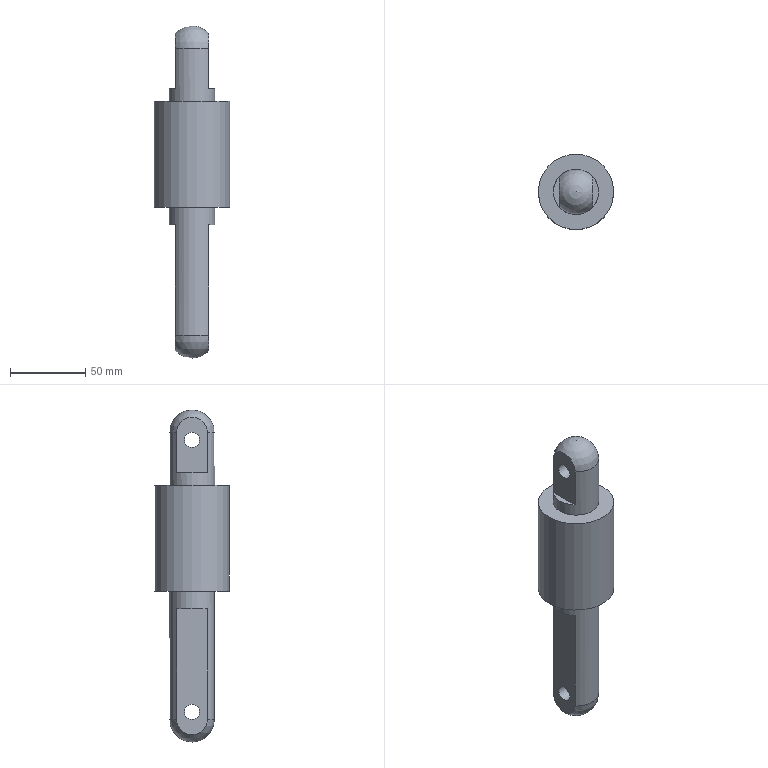Part | NX | features DATUM_CSYS 6, EXTRUDE 5, SKETCH 5, BLEND 2 | 1 solid | 17 faces | box 50 x 50 x 220 mm | volume 220357 mm3 | plane 10 | cylinder 5 | sphere 2 | commonest cylinder face diameters 10 x2 30 x2 50 x1
STEP:
#1=CARTESIAN_POINT('',(15.,0.,100.));
#2=VERTEX_POINT('',#1);
#3=CARTESIAN_POINT('',(0.,0.,100.));
#4=DIRECTION('',(0.,0.,1.));
#5=DIRECTION('',(1.,0.,0.));
#6=AXIS2_PLACEMENT_3D('',#3,#4,#5);
#7=CIRCLE('',#6,15.);
#8=EDGE_CURVE('',#2,#2,#7,.T.);
#9=ORIENTED_EDGE('',*,*,#8,.F.);
#10=EDGE_LOOP('',(#9));
#11=FACE_BOUND('',#10,.T.);
#12=CARTESIAN_POINT('',(11.,10.198,15.));
#13=VERTEX_POINT('',#12);
#14=CARTESIAN_POINT('',(11.,10.198,88.444));
#15=VERTEX_POINT('',#14);
#16=CARTESIAN_POINT('',(11.,10.198,100.));
#17=DIRECTION('',(0.,0.,-1.));
#18=VECTOR('',#17,1000.);
#19=LINE('',#16,#18);
#20=EDGE_CURVE('',#13,#15,#19,.F.);
#21=ORIENTED_EDGE('',*,*,#20,.F.);
#22=CARTESIAN_POINT('',(-11.,10.198,15.));
#23=VERTEX_POINT('',#22);
#24=CARTESIAN_POINT('',(0.,0.,15.));
#25=DIRECTION('',(0.,0.,-1.));
#26=DIRECTION('',(-1.,0.,0.));
#27=AXIS2_PLACEMENT_3D('',#24,#25,#26);
#28=CIRCLE('',#27,15.);
#29=EDGE_CURVE('',#13,#23,#28,.F.);
#30=ORIENTED_EDGE('',*,*,#29,.T.);
#31=CARTESIAN_POINT('',(-11.,10.198,88.444));
#32=VERTEX_POINT('',#31);
#33=CARTESIAN_POINT('',(-11.,10.198,100.));
#34=DIRECTION('',(0.,0.,-1.));
#35=VECTOR('',#34,1000.);
#36=LINE('',#33,#35);
#37=EDGE_CURVE('',#32,#23,#36,.T.);
#38=ORIENTED_EDGE('',*,*,#37,.F.);
#39=CARTESIAN_POINT('',(-11.,-10.198,88.444));
#40=VERTEX_POINT('',#39);
#41=CARTESIAN_POINT('',(0.,0.,88.444));
#42=DIRECTION('',(0.,0.,-1.));
#43=DIRECTION('',(-1.,0.,0.));
#44=AXIS2_PLACEMENT_3D('',#41,#42,#43);
#45=CIRCLE('',#44,15.);
#46=EDGE_CURVE('',#40,#32,#45,.T.);
#47=ORIENTED_EDGE('',*,*,#46,.F.);
#48=CARTESIAN_POINT('',(-11.,-10.198,15.));
#49=VERTEX_POINT('',#48);
#50=CARTESIAN_POINT('',(-11.,-10.198,100.));
#51=DIRECTION('',(0.,0.,-1.));
#52=VECTOR('',#51,1000.);
#53=LINE('',#50,#52);
#54=EDGE_CURVE('',#49,#40,#53,.F.);
#55=ORIENTED_EDGE('',*,*,#54,.F.);
#56=CARTESIAN_POINT('',(11.,-10.198,15.));
#57=VERTEX_POINT('',#56);
#58=CARTESIAN_POINT('',(0.,0.,15.));
#59=DIRECTION('',(0.,0.,-1.));
#60=DIRECTION('',(-1.,0.,0.));
#61=AXIS2_PLACEMENT_3D('',#58,#59,#60);
#62=CIRCLE('',#61,15.);
#63=EDGE_CURVE('',#49,#57,#62,.F.);
#64=ORIENTED_EDGE('',*,*,#63,.T.);
#65=CARTESIAN_POINT('',(11.,-10.198,88.444));
#66=VERTEX_POINT('',#65);
#67=CARTESIAN_POINT('',(11.,-10.198,100.));
#68=DIRECTION('',(0.,0.,-1.));
#69=VECTOR('',#68,1000.);
#70=LINE('',#67,#69);
#71=EDGE_CURVE('',#66,#57,#70,.T.);
#72=ORIENTED_EDGE('',*,*,#71,.F.);
#73=CARTESIAN_POINT('',(0.,0.,88.444));
#74=DIRECTION('',(0.,0.,-1.));
#75=DIRECTION('',(-1.,0.,0.));
#76=AXIS2_PLACEMENT_3D('',#73,#74,#75);
#77=CIRCLE('',#76,15.);
#78=EDGE_CURVE('',#15,#66,#77,.T.);
#79=ORIENTED_EDGE('',*,*,#78,.F.);
#80=EDGE_LOOP('',(#21,#30,#38,#47,#55,#64,#72,#79));
#81=FACE_BOUND('',#80,.T.);
#82=CARTESIAN_POINT('',(0.,0.,100.));
#83=DIRECTION('',(0.,0.,-1.));
#84=DIRECTION('',(-1.,0.,0.));
#85=AXIS2_PLACEMENT_3D('',#82,#83,#84);
#86=CYLINDRICAL_SURFACE('',#85,15.);
#87=ADVANCED_FACE('',(#11,#81),#86,.T.);
#88=CARTESIAN_POINT('',(15.,0.,170.));
#89=VERTEX_POINT('',#88);
#90=CARTESIAN_POINT('',(0.,0.,170.));
#91=DIRECTION('',(0.,0.,1.));
#92=DIRECTION('',(1.,0.,0.));
#93=AXIS2_PLACEMENT_3D('',#90,#91,#92);
#94=CIRCLE('',#93,15.);
#95=EDGE_CURVE('',#89,#89,#94,.T.);
#96=ORIENTED_EDGE('',*,*,#95,.T.);
#97=EDGE_LOOP('',(#96));
#98=FACE_BOUND('',#97,.T.);
#99=CARTESIAN_POINT('',(11.,-10.198,205.));
#100=VERTEX_POINT('',#99);
#101=CARTESIAN_POINT('',(11.,-10.198,178.334));
#102=VERTEX_POINT('',#101);
#103=CARTESIAN_POINT('',(11.,-10.198,220.));
#104=DIRECTION('',(0.,0.,-1.));
#105=VECTOR('',#104,1000.);
#106=LINE('',#103,#105);
#107=EDGE_CURVE('',#100,#102,#106,.T.);
#108=ORIENTED_EDGE('',*,*,#107,.F.);
#109=CARTESIAN_POINT('',(-11.,-10.198,205.));
#110=VERTEX_POINT('',#109);
#111=CARTESIAN_POINT('',(0.,0.,205.));
#112=DIRECTION('',(0.,0.,-1.));
#113=DIRECTION('',(-1.,0.,0.));
#114=AXIS2_PLACEMENT_3D('',#111,#112,#113);
#115=CIRCLE('',#114,15.);
#116=EDGE_CURVE('',#100,#110,#115,.T.);
#117=ORIENTED_EDGE('',*,*,#116,.T.);
#118=CARTESIAN_POINT('',(-11.,-10.198,178.334));
#119=VERTEX_POINT('',#118);
#120=CARTESIAN_POINT('',(-11.,-10.198,220.));
#121=DIRECTION('',(0.,0.,-1.));
#122=VECTOR('',#121,1000.);
#123=LINE('',#120,#122);
#124=EDGE_CURVE('',#119,#110,#123,.F.);
#125=ORIENTED_EDGE('',*,*,#124,.F.);
#126=CARTESIAN_POINT('',(-11.,10.198,178.334));
#127=VERTEX_POINT('',#126);
#128=CARTESIAN_POINT('',(0.,0.,178.334));
#129=DIRECTION('',(0.,0.,1.));
#130=DIRECTION('',(1.,0.,0.));
#131=AXIS2_PLACEMENT_3D('',#128,#129,#130);
#132=CIRCLE('',#131,15.);
#133=EDGE_CURVE('',#127,#119,#132,.T.);
#134=ORIENTED_EDGE('',*,*,#133,.F.);
#135=CARTESIAN_POINT('',(-11.,10.198,205.));
#136=VERTEX_POINT('',#135);
#137=CARTESIAN_POINT('',(-11.,10.198,220.));
#138=DIRECTION('',(0.,0.,-1.));
#139=VECTOR('',#138,1000.);
#140=LINE('',#137,#139);
#141=EDGE_CURVE('',#136,#127,#140,.T.);
#142=ORIENTED_EDGE('',*,*,#141,.F.);
#143=CARTESIAN_POINT('',(11.,10.198,205.));
#144=VERTEX_POINT('',#143);
#145=CARTESIAN_POINT('',(0.,0.,205.));
#146=DIRECTION('',(0.,0.,-1.));
#147=DIRECTION('',(-1.,0.,0.));
#148=AXIS2_PLACEMENT_3D('',#145,#146,#147);
#149=CIRCLE('',#148,15.);
#150=EDGE_CURVE('',#136,#144,#149,.T.);
#151=ORIENTED_EDGE('',*,*,#150,.T.);
#152=CARTESIAN_POINT('',(11.,10.198,178.334));
#153=VERTEX_POINT('',#152);
#154=CARTESIAN_POINT('',(11.,10.198,220.));
#155=DIRECTION('',(0.,0.,-1.));
#156=VECTOR('',#155,1000.);
#157=LINE('',#154,#156);
#158=EDGE_CURVE('',#153,#144,#157,.F.);
#159=ORIENTED_EDGE('',*,*,#158,.F.);
#160=CARTESIAN_POINT('',(0.,0.,178.334));
#161=DIRECTION('',(0.,0.,1.));
#162=DIRECTION('',(1.,0.,0.));
#163=AXIS2_PLACEMENT_3D('',#160,#161,#162);
#164=CIRCLE('',#163,15.);
#165=EDGE_CURVE('',#102,#153,#164,.T.);
#166=ORIENTED_EDGE('',*,*,#165,.F.);
#167=EDGE_LOOP('',(#108,#117,#125,#134,#142,#151,#159,#166));
#168=FACE_BOUND('',#167,.T.);
#169=CARTESIAN_POINT('',(0.,0.,220.));
#170=DIRECTION('',(0.,0.,-1.));
#171=DIRECTION('',(-1.,0.,0.));
#172=AXIS2_PLACEMENT_3D('',#169,#170,#171);
#173=CYLINDRICAL_SURFACE('',#172,15.);
#174=ADVANCED_FACE('',(#98,#168),#173,.T.);
#175=CARTESIAN_POINT('',(25.,0.,170.));
#176=VERTEX_POINT('',#175);
#177=CARTESIAN_POINT('',(0.,0.,170.));
#178=DIRECTION('',(0.,0.,1.));
#179=DIRECTION('',(1.,0.,0.));
#180=AXIS2_PLACEMENT_3D('',#177,#178,#179);
#181=CIRCLE('',#180,25.);
#182=EDGE_CURVE('',#176,#176,#181,.T.);
#183=ORIENTED_EDGE('',*,*,#182,.F.);
#184=EDGE_LOOP('',(#183));
#185=FACE_BOUND('',#184,.T.);
#186=CARTESIAN_POINT('',(25.,0.,100.));
#187=VERTEX_POINT('',#186);
#188=CARTESIAN_POINT('',(0.,0.,100.));
#189=DIRECTION('',(0.,0.,1.));
#190=DIRECTION('',(1.,0.,0.));
#191=AXIS2_PLACEMENT_3D('',#188,#189,#190);
#192=CIRCLE('',#191,25.);
#193=EDGE_CURVE('',#187,#187,#192,.T.);
#194=ORIENTED_EDGE('',*,*,#193,.T.);
#195=EDGE_LOOP('',(#194));
#196=FACE_BOUND('',#195,.T.);
#197=CARTESIAN_POINT('',(0.,0.,170.));
#198=DIRECTION('',(0.,0.,-1.));
#199=DIRECTION('',(-1.,0.,0.));
#200=AXIS2_PLACEMENT_3D('',#197,#198,#199);
#201=CYLINDRICAL_SURFACE('',#200,25.);
#202=ADVANCED_FACE('',(#185,#196),#201,.T.);
#203=ORIENTED_EDGE('',*,*,#95,.F.);
#204=EDGE_LOOP('',(#203));
#205=FACE_BOUND('',#204,.T.);
#206=ORIENTED_EDGE('',*,*,#182,.T.);
#207=EDGE_LOOP('',(#206));
#208=FACE_BOUND('',#207,.T.);
#209=CARTESIAN_POINT('',(0.,0.,170.));
#210=DIRECTION('',(0.,0.,1.));
#211=DIRECTION('',(1.,0.,0.));
#212=AXIS2_PLACEMENT_3D('',#209,#210,#211);
#213=PLANE('',#212);
#214=ADVANCED_FACE('',(#205,#208),#213,.T.);
#215=ORIENTED_EDGE('',*,*,#8,.T.);
#216=EDGE_LOOP('',(#215));
#217=FACE_BOUND('',#216,.T.);
#218=ORIENTED_EDGE('',*,*,#193,.F.);
#219=EDGE_LOOP('',(#218));
#220=FACE_BOUND('',#219,.T.);
#221=CARTESIAN_POINT('',(0.,0.,100.));
#222=DIRECTION('',(0.,0.,1.));
#223=DIRECTION('',(1.,0.,0.));
#224=AXIS2_PLACEMENT_3D('',#221,#222,#223);
#225=PLANE('',#224);
#226=ADVANCED_FACE('',(#217,#220),#225,.F.);
#227=ORIENTED_EDGE('',*,*,#165,.T.);
#228=CARTESIAN_POINT('',(11.,-70.,178.334));
#229=DIRECTION('',(0.,1.,0.));
#230=VECTOR('',#229,1000.);
#231=LINE('',#228,#230);
#232=EDGE_CURVE('',#153,#102,#231,.F.);
#233=ORIENTED_EDGE('',*,*,#232,.T.);
#234=EDGE_LOOP('',(#227,#233));
#235=FACE_BOUND('',#234,.T.);
#236=CARTESIAN_POINT('',(11.,-70.,178.334));
#237=DIRECTION('',(0.,0.,1.));
#238=DIRECTION('',(1.,0.,0.));
#239=AXIS2_PLACEMENT_3D('',#236,#237,#238);
#240=PLANE('',#239);
#241=ADVANCED_FACE('',(#235),#240,.T.);
#242=CARTESIAN_POINT('',(11.,0.,195.198));
#243=VERTEX_POINT('',#242);
#244=CARTESIAN_POINT('',(11.,0.,200.198));
#245=DIRECTION('',(1.,0.,0.));
#246=DIRECTION('',(0.,0.,-1.));
#247=AXIS2_PLACEMENT_3D('',#244,#245,#246);
#248=CIRCLE('',#247,5.);
#249=EDGE_CURVE('',#243,#243,#248,.T.);
#250=ORIENTED_EDGE('',*,*,#249,.F.);
#251=EDGE_LOOP('',(#250));
#252=FACE_BOUND('',#251,.T.);
#253=ORIENTED_EDGE('',*,*,#158,.T.);
#254=CARTESIAN_POINT('',(11.,0.,205.));
#255=DIRECTION('',(1.,0.,0.));
#256=DIRECTION('',(0.,0.,-1.));
#257=AXIS2_PLACEMENT_3D('',#254,#255,#256);
#258=CIRCLE('',#257,10.198);
#259=EDGE_CURVE('',#144,#100,#258,.T.);
#260=ORIENTED_EDGE('',*,*,#259,.T.);
#261=ORIENTED_EDGE('',*,*,#107,.T.);
#262=ORIENTED_EDGE('',*,*,#232,.F.);
#263=EDGE_LOOP('',(#253,#260,#261,#262));
#264=FACE_BOUND('',#263,.T.);
#265=CARTESIAN_POINT('',(11.,-70.,229.55));
#266=DIRECTION('',(1.,0.,0.));
#267=DIRECTION('',(0.,0.,-1.));
#268=AXIS2_PLACEMENT_3D('',#265,#266,#267);
#269=PLANE('',#268);
#270=ADVANCED_FACE('',(#252,#264),#269,.T.);
#271=ORIENTED_EDGE('',*,*,#133,.T.);
#272=CARTESIAN_POINT('',(-11.,-70.,178.334));
#273=DIRECTION('',(0.,1.,0.));
#274=VECTOR('',#273,1000.);
#275=LINE('',#272,#274);
#276=EDGE_CURVE('',#127,#119,#275,.F.);
#277=ORIENTED_EDGE('',*,*,#276,.F.);
#278=EDGE_LOOP('',(#271,#277));
#279=FACE_BOUND('',#278,.T.);
#280=CARTESIAN_POINT('',(-39.37,-70.,178.334));
#281=DIRECTION('',(0.,0.,1.));
#282=DIRECTION('',(1.,0.,0.));
#283=AXIS2_PLACEMENT_3D('',#280,#281,#282);
#284=PLANE('',#283);
#285=ADVANCED_FACE('',(#279),#284,.T.);
#286=CARTESIAN_POINT('',(-11.,0.,205.198));
#287=VERTEX_POINT('',#286);
#288=CARTESIAN_POINT('',(-11.,0.,200.198));
#289=DIRECTION('',(-1.,0.,0.));
#290=DIRECTION('',(0.,0.,1.));
#291=AXIS2_PLACEMENT_3D('',#288,#289,#290);
#292=CIRCLE('',#291,5.);
#293=EDGE_CURVE('',#287,#287,#292,.T.);
#294=ORIENTED_EDGE('',*,*,#293,.F.);
#295=EDGE_LOOP('',(#294));
#296=FACE_BOUND('',#295,.T.);
#297=ORIENTED_EDGE('',*,*,#124,.T.);
#298=CARTESIAN_POINT('',(-11.,0.,205.));
#299=DIRECTION('',(-1.,0.,0.));
#300=DIRECTION('',(0.,0.,1.));
#301=AXIS2_PLACEMENT_3D('',#298,#299,#300);
#302=CIRCLE('',#301,10.198);
#303=EDGE_CURVE('',#110,#136,#302,.T.);
#304=ORIENTED_EDGE('',*,*,#303,.T.);
#305=ORIENTED_EDGE('',*,*,#141,.T.);
#306=ORIENTED_EDGE('',*,*,#276,.T.);
#307=EDGE_LOOP('',(#297,#304,#305,#306));
#308=FACE_BOUND('',#307,.T.);
#309=CARTESIAN_POINT('',(-11.,-70.,178.334));
#310=DIRECTION('',(-1.,0.,0.));
#311=DIRECTION('',(0.,0.,1.));
#312=AXIS2_PLACEMENT_3D('',#309,#310,#311);
#313=PLANE('',#312);
#314=ADVANCED_FACE('',(#296,#308),#313,.T.);
#315=ORIENTED_EDGE('',*,*,#46,.T.);
#316=CARTESIAN_POINT('',(-11.,-70.,88.444));
#317=DIRECTION('',(0.,1.,0.));
#318=VECTOR('',#317,1000.);
#319=LINE('',#316,#318);
#320=EDGE_CURVE('',#32,#40,#319,.F.);
#321=ORIENTED_EDGE('',*,*,#320,.T.);
#322=EDGE_LOOP('',(#315,#321));
#323=FACE_BOUND('',#322,.T.);
#324=CARTESIAN_POINT('',(-11.,-70.,88.444));
#325=DIRECTION('',(0.,0.,-1.));
#326=DIRECTION('',(-1.,0.,0.));
#327=AXIS2_PLACEMENT_3D('',#324,#325,#326);
#328=PLANE('',#327);
#329=ADVANCED_FACE('',(#323),#328,.T.);
#330=CARTESIAN_POINT('',(-11.,0.,25.));
#331=VERTEX_POINT('',#330);
#332=CARTESIAN_POINT('',(-11.,0.,20.));
#333=DIRECTION('',(-1.,0.,0.));
#334=DIRECTION('',(0.,0.,1.));
#335=AXIS2_PLACEMENT_3D('',#332,#333,#334);
#336=CIRCLE('',#335,5.);
#337=EDGE_CURVE('',#331,#331,#336,.T.);
#338=ORIENTED_EDGE('',*,*,#337,.F.);
#339=EDGE_LOOP('',(#338));
#340=FACE_BOUND('',#339,.T.);
#341=ORIENTED_EDGE('',*,*,#37,.T.);
#342=CARTESIAN_POINT('',(-11.,0.,15.));
#343=DIRECTION('',(-1.,0.,0.));
#344=DIRECTION('',(0.,0.,1.));
#345=AXIS2_PLACEMENT_3D('',#342,#343,#344);
#346=CIRCLE('',#345,10.198);
#347=EDGE_CURVE('',#23,#49,#346,.T.);
#348=ORIENTED_EDGE('',*,*,#347,.T.);
#349=ORIENTED_EDGE('',*,*,#54,.T.);
#350=ORIENTED_EDGE('',*,*,#320,.F.);
#351=EDGE_LOOP('',(#341,#348,#349,#350));
#352=FACE_BOUND('',#351,.T.);
#353=CARTESIAN_POINT('',(-11.,-70.,-99.));
#354=DIRECTION('',(-1.,0.,0.));
#355=DIRECTION('',(0.,0.,1.));
#356=AXIS2_PLACEMENT_3D('',#353,#354,#355);
#357=PLANE('',#356);
#358=ADVANCED_FACE('',(#340,#352),#357,.T.);
#359=ORIENTED_EDGE('',*,*,#78,.T.);
#360=CARTESIAN_POINT('',(11.,-70.,88.444));
#361=DIRECTION('',(0.,1.,0.));
#362=VECTOR('',#361,1000.);
#363=LINE('',#360,#362);
#364=EDGE_CURVE('',#15,#66,#363,.F.);
#365=ORIENTED_EDGE('',*,*,#364,.F.);
#366=EDGE_LOOP('',(#359,#365));
#367=FACE_BOUND('',#366,.T.);
#368=CARTESIAN_POINT('',(72.429,-70.,88.444));
#369=DIRECTION('',(0.,0.,-1.));
#370=DIRECTION('',(-1.,0.,0.));
#371=AXIS2_PLACEMENT_3D('',#368,#369,#370);
#372=PLANE('',#371);
#373=ADVANCED_FACE('',(#367),#372,.T.);
#374=CARTESIAN_POINT('',(11.,0.,15.));
#375=VERTEX_POINT('',#374);
#376=CARTESIAN_POINT('',(11.,0.,20.));
#377=DIRECTION('',(1.,0.,0.));
#378=DIRECTION('',(0.,0.,-1.));
#379=AXIS2_PLACEMENT_3D('',#376,#377,#378);
#380=CIRCLE('',#379,5.);
#381=EDGE_CURVE('',#375,#375,#380,.T.);
#382=ORIENTED_EDGE('',*,*,#381,.F.);
#383=EDGE_LOOP('',(#382));
#384=FACE_BOUND('',#383,.T.);
#385=ORIENTED_EDGE('',*,*,#71,.T.);
#386=CARTESIAN_POINT('',(11.,0.,15.));
#387=DIRECTION('',(1.,0.,0.));
#388=DIRECTION('',(0.,0.,-1.));
#389=AXIS2_PLACEMENT_3D('',#386,#387,#388);
#390=CIRCLE('',#389,10.198);
#391=EDGE_CURVE('',#57,#13,#390,.T.);
#392=ORIENTED_EDGE('',*,*,#391,.T.);
#393=ORIENTED_EDGE('',*,*,#20,.T.);
#394=ORIENTED_EDGE('',*,*,#364,.T.);
#395=EDGE_LOOP('',(#385,#392,#393,#394));
#396=FACE_BOUND('',#395,.T.);
#397=CARTESIAN_POINT('',(11.,-70.,88.444));
#398=DIRECTION('',(1.,0.,0.));
#399=DIRECTION('',(0.,0.,-1.));
#400=AXIS2_PLACEMENT_3D('',#397,#398,#399);
#401=PLANE('',#400);
#402=ADVANCED_FACE('',(#384,#396),#401,.T.);
#403=ORIENTED_EDGE('',*,*,#347,.F.);
#404=ORIENTED_EDGE('',*,*,#29,.F.);
#405=ORIENTED_EDGE('',*,*,#391,.F.);
#406=ORIENTED_EDGE('',*,*,#63,.F.);
#407=EDGE_LOOP('',(#403,#404,#405,#406));
#408=FACE_BOUND('',#407,.T.);
#409=CARTESIAN_POINT('',(0.,0.,15.));
#410=DIRECTION('',(0.,0.,1.));
#411=DIRECTION('',(1.,0.,0.));
#412=AXIS2_PLACEMENT_3D('',#409,#410,#411);
#413=SPHERICAL_SURFACE('',#412,15.);
#414=ADVANCED_FACE('',(#408),#413,.T.);
#415=ORIENTED_EDGE('',*,*,#303,.F.);
#416=ORIENTED_EDGE('',*,*,#116,.F.);
#417=ORIENTED_EDGE('',*,*,#259,.F.);
#418=ORIENTED_EDGE('',*,*,#150,.F.);
#419=EDGE_LOOP('',(#415,#416,#417,#418));
#420=FACE_BOUND('',#419,.T.);
#421=CARTESIAN_POINT('',(0.,0.,205.));
#422=DIRECTION('',(0.,0.,1.));
#423=DIRECTION('',(1.,0.,0.));
#424=AXIS2_PLACEMENT_3D('',#421,#422,#423);
#425=SPHERICAL_SURFACE('',#424,15.);
#426=ADVANCED_FACE('',(#420),#425,.T.);
#427=ORIENTED_EDGE('',*,*,#337,.T.);
#428=EDGE_LOOP('',(#427));
#429=FACE_BOUND('',#428,.T.);
#430=ORIENTED_EDGE('',*,*,#381,.T.);
#431=EDGE_LOOP('',(#430));
#432=FACE_BOUND('',#431,.T.);
#433=CARTESIAN_POINT('',(-74.,0.,20.));
#434=DIRECTION('',(1.,0.,0.));
#435=DIRECTION('',(0.,0.,-1.));
#436=AXIS2_PLACEMENT_3D('',#433,#434,#435);
#437=CYLINDRICAL_SURFACE('',#436,5.);
#438=ADVANCED_FACE('',(#429,#432),#437,.F.);
#439=ORIENTED_EDGE('',*,*,#293,.T.);
#440=EDGE_LOOP('',(#439));
#441=FACE_BOUND('',#440,.T.);
#442=ORIENTED_EDGE('',*,*,#249,.T.);
#443=EDGE_LOOP('',(#442));
#444=FACE_BOUND('',#443,.T.);
#445=CARTESIAN_POINT('',(-74.,0.,200.198));
#446=DIRECTION('',(1.,0.,0.));
#447=DIRECTION('',(0.,0.,-1.));
#448=AXIS2_PLACEMENT_3D('',#445,#446,#447);
#449=CYLINDRICAL_SURFACE('',#448,5.);
#450=ADVANCED_FACE('',(#441,#444),#449,.F.);
#451=CLOSED_SHELL('',(#87,#174,#202,#214,#226,#241,#270,#285,#314,#329,#358,#373,#402,#414,#426,#438,#450));
#452=MANIFOLD_SOLID_BREP('',#451);
#453=(LENGTH_UNIT()NAMED_UNIT(*)SI_UNIT(.MILLI.,.METRE.));
#454=UNCERTAINTY_MEASURE_WITH_UNIT(LENGTH_MEASURE(0.00001),#453,'','');
#455=(NAMED_UNIT(*)PLANE_ANGLE_UNIT()SI_UNIT($,.RADIAN.));
#456=(NAMED_UNIT(*)SI_UNIT($,.STERADIAN.)SOLID_ANGLE_UNIT());
#457=(GEOMETRIC_REPRESENTATION_CONTEXT(3)GLOBAL_UNCERTAINTY_ASSIGNED_CONTEXT((#454))GLOBAL_UNIT_ASSIGNED_CONTEXT((#453,#455,#456))REPRESENTATION_CONTEXT('',''));
#458=ADVANCED_BREP_SHAPE_REPRESENTATION('',(#452),#457);